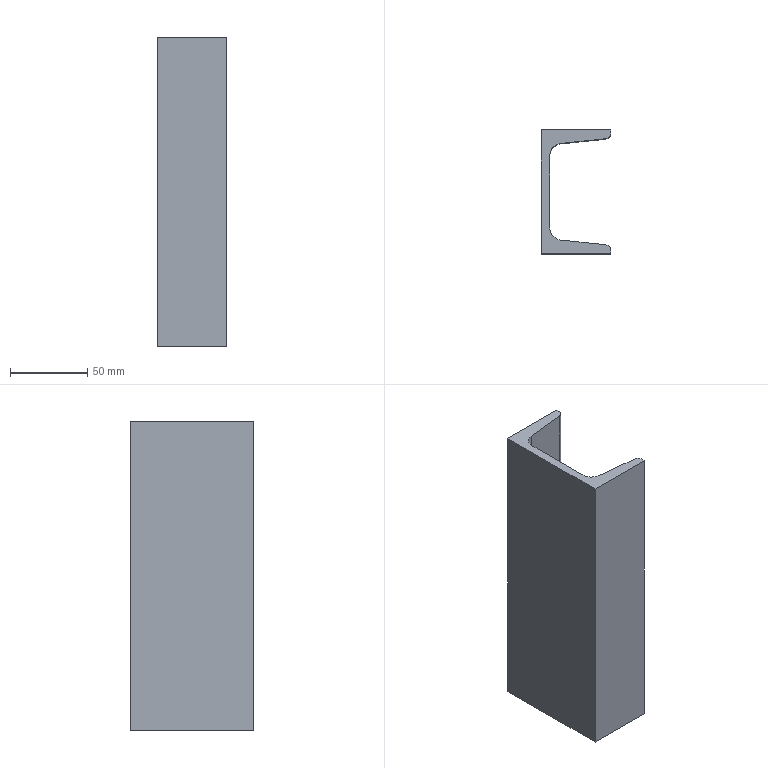Part | STEP file | ISO 657_11 CH 80 x 8 1784900614284 | 1 solid | 14 faces | box 45 x 80 x 200 mm | volume 209713 mm3 | plane 10 | cylinder 4 | commonest cylinder face diameters 8 x2 16 x2
STEP:
#1=CARTESIAN_POINT('',(4.07,-23.221,200.));
#2=VERTEX_POINT('',#1);
#3=CARTESIAN_POINT('',(11.234,-31.177,200.));
#4=VERTEX_POINT('',#3);
#5=CARTESIAN_POINT('',(12.07,-23.221,200.));
#6=DIRECTION('',(0.,0.,1.));
#7=DIRECTION('',(-1.,0.,0.));
#8=AXIS2_PLACEMENT_3D('',#5,#6,#7);
#9=CIRCLE('',#8,8.);
#10=EDGE_CURVE('',#2,#4,#9,.T.);
#11=ORIENTED_EDGE('',*,*,#10,.T.);
#12=CARTESIAN_POINT('',(11.234,-31.177,0.));
#13=VERTEX_POINT('',#12);
#14=CARTESIAN_POINT('',(11.234,-31.177,0.));
#15=DIRECTION('',(0.,0.,1.));
#16=VECTOR('',#15,10.);
#17=LINE('',#14,#16);
#18=EDGE_CURVE('',#13,#4,#17,.T.);
#19=ORIENTED_EDGE('',*,*,#18,.F.);
#20=CARTESIAN_POINT('',(4.07,-23.221,0.));
#21=VERTEX_POINT('',#20);
#22=CARTESIAN_POINT('',(12.07,-23.221,0.));
#23=DIRECTION('',(0.,0.,1.));
#24=DIRECTION('',(-1.,0.,0.));
#25=AXIS2_PLACEMENT_3D('',#22,#23,#24);
#26=CIRCLE('',#25,8.);
#27=EDGE_CURVE('',#21,#13,#26,.T.);
#28=ORIENTED_EDGE('',*,*,#27,.F.);
#29=CARTESIAN_POINT('',(4.07,-23.221,0.));
#30=DIRECTION('',(0.,0.,1.));
#31=VECTOR('',#30,10.);
#32=LINE('',#29,#31);
#33=EDGE_CURVE('',#21,#2,#32,.T.);
#34=ORIENTED_EDGE('',*,*,#33,.T.);
#35=EDGE_LOOP('',(#11,#19,#28,#34));
#36=FACE_OUTER_BOUND('',#35,.T.);
#37=CARTESIAN_POINT('',(12.07,-23.221,0.));
#38=DIRECTION('',(0.,0.,1.));
#39=DIRECTION('',(-1.,0.,0.));
#40=AXIS2_PLACEMENT_3D('',#37,#38,#39);
#41=CYLINDRICAL_SURFACE('',#40,8.);
#42=ADVANCED_FACE('',(#36),#41,.F.);
#43=CARTESIAN_POINT('',(39.988,-34.199,200.));
#44=VERTEX_POINT('',#43);
#45=CARTESIAN_POINT('',(14.478,-31.518,200.));
#46=DIRECTION('',(0.9945,-0.1045,0.));
#47=VECTOR('',#46,10.);
#48=LINE('',#45,#47);
#49=EDGE_CURVE('',#4,#44,#48,.T.);
#50=ORIENTED_EDGE('',*,*,#49,.T.);
#51=CARTESIAN_POINT('',(39.988,-34.199,0.));
#52=VERTEX_POINT('',#51);
#53=CARTESIAN_POINT('',(39.988,-34.199,0.));
#54=DIRECTION('',(0.,0.,1.));
#55=VECTOR('',#54,10.);
#56=LINE('',#53,#55);
#57=EDGE_CURVE('',#52,#44,#56,.T.);
#58=ORIENTED_EDGE('',*,*,#57,.F.);
#59=CARTESIAN_POINT('',(14.478,-31.518,0.));
#60=DIRECTION('',(0.9945,-0.1045,0.));
#61=VECTOR('',#60,10.);
#62=LINE('',#59,#61);
#63=EDGE_CURVE('',#13,#52,#62,.T.);
#64=ORIENTED_EDGE('',*,*,#63,.F.);
#65=ORIENTED_EDGE('',*,*,#18,.T.);
#66=EDGE_LOOP('',(#50,#58,#64,#65));
#67=FACE_OUTER_BOUND('',#66,.T.);
#68=CARTESIAN_POINT('',(11.234,-31.177,0.));
#69=DIRECTION('',(0.1045,0.9945,0.));
#70=DIRECTION('',(0.,0.,1.));
#71=AXIS2_PLACEMENT_3D('',#68,#69,#70);
#72=PLANE('',#71);
#73=ADVANCED_FACE('',(#67),#72,.T.);
#74=CARTESIAN_POINT('',(43.57,-38.177,200.));
#75=VERTEX_POINT('',#74);
#76=CARTESIAN_POINT('',(39.57,-38.177,200.));
#77=DIRECTION('',(0.,0.,-1.));
#78=DIRECTION('',(-1.,0.,0.));
#79=AXIS2_PLACEMENT_3D('',#76,#77,#78);
#80=CIRCLE('',#79,4.);
#81=EDGE_CURVE('',#44,#75,#80,.T.);
#82=ORIENTED_EDGE('',*,*,#81,.T.);
#83=CARTESIAN_POINT('',(43.57,-38.177,0.));
#84=VERTEX_POINT('',#83);
#85=CARTESIAN_POINT('',(43.57,-38.177,0.));
#86=DIRECTION('',(0.,0.,1.));
#87=VECTOR('',#86,10.);
#88=LINE('',#85,#87);
#89=EDGE_CURVE('',#84,#75,#88,.T.);
#90=ORIENTED_EDGE('',*,*,#89,.F.);
#91=CARTESIAN_POINT('',(39.57,-38.177,0.));
#92=DIRECTION('',(0.,0.,-1.));
#93=DIRECTION('',(-1.,0.,0.));
#94=AXIS2_PLACEMENT_3D('',#91,#92,#93);
#95=CIRCLE('',#94,4.);
#96=EDGE_CURVE('',#52,#84,#95,.T.);
#97=ORIENTED_EDGE('',*,*,#96,.F.);
#98=ORIENTED_EDGE('',*,*,#57,.T.);
#99=EDGE_LOOP('',(#82,#90,#97,#98));
#100=FACE_OUTER_BOUND('',#99,.T.);
#101=CARTESIAN_POINT('',(39.57,-38.177,0.));
#102=DIRECTION('',(0.,0.,1.));
#103=DIRECTION('',(-1.,0.,0.));
#104=AXIS2_PLACEMENT_3D('',#101,#102,#103);
#105=CYLINDRICAL_SURFACE('',#104,4.);
#106=ADVANCED_FACE('',(#100),#105,.T.);
#107=CARTESIAN_POINT('',(43.57,-40.,200.));
#108=VERTEX_POINT('',#107);
#109=CARTESIAN_POINT('',(43.57,-19.089,200.));
#110=DIRECTION('',(0.,-1.,0.));
#111=VECTOR('',#110,10.);
#112=LINE('',#109,#111);
#113=EDGE_CURVE('',#75,#108,#112,.T.);
#114=ORIENTED_EDGE('',*,*,#113,.T.);
#115=CARTESIAN_POINT('',(43.57,-40.,0.));
#116=VERTEX_POINT('',#115);
#117=CARTESIAN_POINT('',(43.57,-40.,0.));
#118=DIRECTION('',(0.,0.,1.));
#119=VECTOR('',#118,10.);
#120=LINE('',#117,#119);
#121=EDGE_CURVE('',#116,#108,#120,.T.);
#122=ORIENTED_EDGE('',*,*,#121,.F.);
#123=CARTESIAN_POINT('',(43.57,-19.089,0.));
#124=DIRECTION('',(0.,-1.,0.));
#125=VECTOR('',#124,10.);
#126=LINE('',#123,#125);
#127=EDGE_CURVE('',#84,#116,#126,.T.);
#128=ORIENTED_EDGE('',*,*,#127,.F.);
#129=ORIENTED_EDGE('',*,*,#89,.T.);
#130=EDGE_LOOP('',(#114,#122,#128,#129));
#131=FACE_OUTER_BOUND('',#130,.T.);
#132=CARTESIAN_POINT('',(43.57,-38.177,0.));
#133=DIRECTION('',(1.,0.,0.));
#134=DIRECTION('',(0.,0.,-1.));
#135=AXIS2_PLACEMENT_3D('',#132,#133,#134);
#136=PLANE('',#135);
#137=ADVANCED_FACE('',(#131),#136,.T.);
#138=CARTESIAN_POINT('',(-1.43,-40.,200.));
#139=VERTEX_POINT('',#138);
#140=CARTESIAN_POINT('',(32.32,-40.,200.));
#141=DIRECTION('',(-1.,0.,0.));
#142=VECTOR('',#141,10.);
#143=LINE('',#140,#142);
#144=EDGE_CURVE('',#108,#139,#143,.T.);
#145=ORIENTED_EDGE('',*,*,#144,.T.);
#146=CARTESIAN_POINT('',(-1.43,-40.,0.));
#147=VERTEX_POINT('',#146);
#148=CARTESIAN_POINT('',(-1.43,-40.,0.));
#149=DIRECTION('',(0.,0.,1.));
#150=VECTOR('',#149,10.);
#151=LINE('',#148,#150);
#152=EDGE_CURVE('',#147,#139,#151,.T.);
#153=ORIENTED_EDGE('',*,*,#152,.F.);
#154=CARTESIAN_POINT('',(32.32,-40.,0.));
#155=DIRECTION('',(-1.,0.,0.));
#156=VECTOR('',#155,10.);
#157=LINE('',#154,#156);
#158=EDGE_CURVE('',#116,#147,#157,.T.);
#159=ORIENTED_EDGE('',*,*,#158,.F.);
#160=ORIENTED_EDGE('',*,*,#121,.T.);
#161=EDGE_LOOP('',(#145,#153,#159,#160));
#162=FACE_OUTER_BOUND('',#161,.T.);
#163=CARTESIAN_POINT('',(43.57,-40.,0.));
#164=DIRECTION('',(0.,-1.,0.));
#165=DIRECTION('',(0.,0.,-1.));
#166=AXIS2_PLACEMENT_3D('',#163,#164,#165);
#167=PLANE('',#166);
#168=ADVANCED_FACE('',(#162),#167,.T.);
#169=CARTESIAN_POINT('',(-1.43,40.,200.));
#170=VERTEX_POINT('',#169);
#171=CARTESIAN_POINT('',(-1.43,0.,200.));
#172=DIRECTION('',(0.,1.,0.));
#173=VECTOR('',#172,10.);
#174=LINE('',#171,#173);
#175=EDGE_CURVE('',#139,#170,#174,.T.);
#176=ORIENTED_EDGE('',*,*,#175,.T.);
#177=CARTESIAN_POINT('',(-1.43,40.,0.));
#178=VERTEX_POINT('',#177);
#179=CARTESIAN_POINT('',(-1.43,40.,0.));
#180=DIRECTION('',(0.,0.,1.));
#181=VECTOR('',#180,10.);
#182=LINE('',#179,#181);
#183=EDGE_CURVE('',#178,#170,#182,.T.);
#184=ORIENTED_EDGE('',*,*,#183,.F.);
#185=CARTESIAN_POINT('',(-1.43,0.,0.));
#186=DIRECTION('',(0.,1.,0.));
#187=VECTOR('',#186,10.);
#188=LINE('',#185,#187);
#189=EDGE_CURVE('',#147,#178,#188,.T.);
#190=ORIENTED_EDGE('',*,*,#189,.F.);
#191=ORIENTED_EDGE('',*,*,#152,.T.);
#192=EDGE_LOOP('',(#176,#184,#190,#191));
#193=FACE_OUTER_BOUND('',#192,.T.);
#194=CARTESIAN_POINT('',(-1.43,0.,0.));
#195=DIRECTION('',(-1.,0.,0.));
#196=DIRECTION('',(0.,0.,1.));
#197=AXIS2_PLACEMENT_3D('',#194,#195,#196);
#198=PLANE('',#197);
#199=ADVANCED_FACE('',(#193),#198,.T.);
#200=CARTESIAN_POINT('',(43.57,40.,200.));
#201=VERTEX_POINT('',#200);
#202=CARTESIAN_POINT('',(9.82,40.,200.));
#203=DIRECTION('',(1.,0.,0.));
#204=VECTOR('',#203,10.);
#205=LINE('',#202,#204);
#206=EDGE_CURVE('',#170,#201,#205,.T.);
#207=ORIENTED_EDGE('',*,*,#206,.T.);
#208=CARTESIAN_POINT('',(43.57,40.,0.));
#209=VERTEX_POINT('',#208);
#210=CARTESIAN_POINT('',(43.57,40.,0.));
#211=DIRECTION('',(0.,0.,1.));
#212=VECTOR('',#211,10.);
#213=LINE('',#210,#212);
#214=EDGE_CURVE('',#209,#201,#213,.T.);
#215=ORIENTED_EDGE('',*,*,#214,.F.);
#216=CARTESIAN_POINT('',(9.82,40.,0.));
#217=DIRECTION('',(1.,0.,0.));
#218=VECTOR('',#217,10.);
#219=LINE('',#216,#218);
#220=EDGE_CURVE('',#178,#209,#219,.T.);
#221=ORIENTED_EDGE('',*,*,#220,.F.);
#222=ORIENTED_EDGE('',*,*,#183,.T.);
#223=EDGE_LOOP('',(#207,#215,#221,#222));
#224=FACE_OUTER_BOUND('',#223,.T.);
#225=CARTESIAN_POINT('',(-1.43,40.,0.));
#226=DIRECTION('',(0.,1.,0.));
#227=DIRECTION('',(0.,0.,1.));
#228=AXIS2_PLACEMENT_3D('',#225,#226,#227);
#229=PLANE('',#228);
#230=ADVANCED_FACE('',(#224),#229,.T.);
#231=CARTESIAN_POINT('',(43.57,38.177,200.));
#232=VERTEX_POINT('',#231);
#233=CARTESIAN_POINT('',(43.57,20.,200.));
#234=DIRECTION('',(0.,-1.,0.));
#235=VECTOR('',#234,10.);
#236=LINE('',#233,#235);
#237=EDGE_CURVE('',#201,#232,#236,.T.);
#238=ORIENTED_EDGE('',*,*,#237,.T.);
#239=CARTESIAN_POINT('',(43.57,38.177,0.));
#240=VERTEX_POINT('',#239);
#241=CARTESIAN_POINT('',(43.57,38.177,0.));
#242=DIRECTION('',(0.,0.,1.));
#243=VECTOR('',#242,10.);
#244=LINE('',#241,#243);
#245=EDGE_CURVE('',#240,#232,#244,.T.);
#246=ORIENTED_EDGE('',*,*,#245,.F.);
#247=CARTESIAN_POINT('',(43.57,20.,0.));
#248=DIRECTION('',(0.,-1.,0.));
#249=VECTOR('',#248,10.);
#250=LINE('',#247,#249);
#251=EDGE_CURVE('',#209,#240,#250,.T.);
#252=ORIENTED_EDGE('',*,*,#251,.F.);
#253=ORIENTED_EDGE('',*,*,#214,.T.);
#254=EDGE_LOOP('',(#238,#246,#252,#253));
#255=FACE_OUTER_BOUND('',#254,.T.);
#256=CARTESIAN_POINT('',(43.57,40.,0.));
#257=DIRECTION('',(1.,0.,0.));
#258=DIRECTION('',(0.,0.,-1.));
#259=AXIS2_PLACEMENT_3D('',#256,#257,#258);
#260=PLANE('',#259);
#261=ADVANCED_FACE('',(#255),#260,.T.);
#262=CARTESIAN_POINT('',(39.988,34.199,200.));
#263=VERTEX_POINT('',#262);
#264=CARTESIAN_POINT('',(39.57,38.177,200.));
#265=DIRECTION('',(0.,0.,-1.));
#266=DIRECTION('',(-0.1045,0.9945,0.));
#267=AXIS2_PLACEMENT_3D('',#264,#265,#266);
#268=CIRCLE('',#267,4.);
#269=EDGE_CURVE('',#232,#263,#268,.T.);
#270=ORIENTED_EDGE('',*,*,#269,.T.);
#271=CARTESIAN_POINT('',(39.988,34.199,0.));
#272=VERTEX_POINT('',#271);
#273=CARTESIAN_POINT('',(39.988,34.199,0.));
#274=DIRECTION('',(0.,0.,1.));
#275=VECTOR('',#274,10.);
#276=LINE('',#273,#275);
#277=EDGE_CURVE('',#272,#263,#276,.T.);
#278=ORIENTED_EDGE('',*,*,#277,.F.);
#279=CARTESIAN_POINT('',(39.57,38.177,0.));
#280=DIRECTION('',(0.,0.,-1.));
#281=DIRECTION('',(-0.1045,0.9945,0.));
#282=AXIS2_PLACEMENT_3D('',#279,#280,#281);
#283=CIRCLE('',#282,4.);
#284=EDGE_CURVE('',#240,#272,#283,.T.);
#285=ORIENTED_EDGE('',*,*,#284,.F.);
#286=ORIENTED_EDGE('',*,*,#245,.T.);
#287=EDGE_LOOP('',(#270,#278,#285,#286));
#288=FACE_OUTER_BOUND('',#287,.T.);
#289=CARTESIAN_POINT('',(39.57,38.177,0.));
#290=DIRECTION('',(0.,0.,1.));
#291=DIRECTION('',(-0.1045,0.9945,0.));
#292=AXIS2_PLACEMENT_3D('',#289,#290,#291);
#293=CYLINDRICAL_SURFACE('',#292,4.);
#294=ADVANCED_FACE('',(#288),#293,.T.);
#295=CARTESIAN_POINT('',(11.234,31.177,200.));
#296=VERTEX_POINT('',#295);
#297=CARTESIAN_POINT('',(28.855,33.029,200.));
#298=DIRECTION('',(-0.9945,-0.1045,0.));
#299=VECTOR('',#298,10.);
#300=LINE('',#297,#299);
#301=EDGE_CURVE('',#263,#296,#300,.T.);
#302=ORIENTED_EDGE('',*,*,#301,.T.);
#303=CARTESIAN_POINT('',(11.234,31.177,0.));
#304=VERTEX_POINT('',#303);
#305=CARTESIAN_POINT('',(11.234,31.177,0.));
#306=DIRECTION('',(0.,0.,1.));
#307=VECTOR('',#306,10.);
#308=LINE('',#305,#307);
#309=EDGE_CURVE('',#304,#296,#308,.T.);
#310=ORIENTED_EDGE('',*,*,#309,.F.);
#311=CARTESIAN_POINT('',(28.855,33.029,0.));
#312=DIRECTION('',(-0.9945,-0.1045,0.));
#313=VECTOR('',#312,10.);
#314=LINE('',#311,#313);
#315=EDGE_CURVE('',#272,#304,#314,.T.);
#316=ORIENTED_EDGE('',*,*,#315,.F.);
#317=ORIENTED_EDGE('',*,*,#277,.T.);
#318=EDGE_LOOP('',(#302,#310,#316,#317));
#319=FACE_OUTER_BOUND('',#318,.T.);
#320=CARTESIAN_POINT('',(39.988,34.199,0.));
#321=DIRECTION('',(0.1045,-0.9945,0.));
#322=DIRECTION('',(0.,0.,-1.));
#323=AXIS2_PLACEMENT_3D('',#320,#321,#322);
#324=PLANE('',#323);
#325=ADVANCED_FACE('',(#319),#324,.T.);
#326=CARTESIAN_POINT('',(4.07,23.221,200.));
#327=VERTEX_POINT('',#326);
#328=CARTESIAN_POINT('',(12.07,23.221,200.));
#329=DIRECTION('',(0.,0.,1.));
#330=DIRECTION('',(-0.1045,0.9945,0.));
#331=AXIS2_PLACEMENT_3D('',#328,#329,#330);
#332=CIRCLE('',#331,8.);
#333=EDGE_CURVE('',#296,#327,#332,.T.);
#334=ORIENTED_EDGE('',*,*,#333,.T.);
#335=CARTESIAN_POINT('',(4.07,23.221,0.));
#336=VERTEX_POINT('',#335);
#337=CARTESIAN_POINT('',(4.07,23.221,0.));
#338=DIRECTION('',(0.,0.,1.));
#339=VECTOR('',#338,10.);
#340=LINE('',#337,#339);
#341=EDGE_CURVE('',#336,#327,#340,.T.);
#342=ORIENTED_EDGE('',*,*,#341,.F.);
#343=CARTESIAN_POINT('',(12.07,23.221,0.));
#344=DIRECTION('',(0.,0.,1.));
#345=DIRECTION('',(-0.1045,0.9945,0.));
#346=AXIS2_PLACEMENT_3D('',#343,#344,#345);
#347=CIRCLE('',#346,8.);
#348=EDGE_CURVE('',#304,#336,#347,.T.);
#349=ORIENTED_EDGE('',*,*,#348,.F.);
#350=ORIENTED_EDGE('',*,*,#309,.T.);
#351=EDGE_LOOP('',(#334,#342,#349,#350));
#352=FACE_OUTER_BOUND('',#351,.T.);
#353=CARTESIAN_POINT('',(12.07,23.221,0.));
#354=DIRECTION('',(0.,0.,1.));
#355=DIRECTION('',(-0.1045,0.9945,0.));
#356=AXIS2_PLACEMENT_3D('',#353,#354,#355);
#357=CYLINDRICAL_SURFACE('',#356,8.);
#358=ADVANCED_FACE('',(#352),#357,.F.);
#359=CARTESIAN_POINT('',(4.07,0.,200.));
#360=DIRECTION('',(0.,-1.,0.));
#361=VECTOR('',#360,10.);
#362=LINE('',#359,#361);
#363=EDGE_CURVE('',#327,#2,#362,.T.);
#364=ORIENTED_EDGE('',*,*,#363,.T.);
#365=ORIENTED_EDGE('',*,*,#33,.F.);
#366=CARTESIAN_POINT('',(4.07,0.,0.));
#367=DIRECTION('',(0.,-1.,0.));
#368=VECTOR('',#367,10.);
#369=LINE('',#366,#368);
#370=EDGE_CURVE('',#336,#21,#369,.T.);
#371=ORIENTED_EDGE('',*,*,#370,.F.);
#372=ORIENTED_EDGE('',*,*,#341,.T.);
#373=EDGE_LOOP('',(#364,#365,#371,#372));
#374=FACE_OUTER_BOUND('',#373,.T.);
#375=CARTESIAN_POINT('',(4.07,0.,0.));
#376=DIRECTION('',(1.,0.,0.));
#377=DIRECTION('',(0.,0.,-1.));
#378=AXIS2_PLACEMENT_3D('',#375,#376,#377);
#379=PLANE('',#378);
#380=ADVANCED_FACE('',(#374),#379,.T.);
#381=ORIENTED_EDGE('',*,*,#220,.T.);
#382=ORIENTED_EDGE('',*,*,#251,.T.);
#383=ORIENTED_EDGE('',*,*,#284,.T.);
#384=ORIENTED_EDGE('',*,*,#315,.T.);
#385=ORIENTED_EDGE('',*,*,#348,.T.);
#386=ORIENTED_EDGE('',*,*,#370,.T.);
#387=ORIENTED_EDGE('',*,*,#27,.T.);
#388=ORIENTED_EDGE('',*,*,#63,.T.);
#389=ORIENTED_EDGE('',*,*,#96,.T.);
#390=ORIENTED_EDGE('',*,*,#127,.T.);
#391=ORIENTED_EDGE('',*,*,#158,.T.);
#392=ORIENTED_EDGE('',*,*,#189,.T.);
#393=EDGE_LOOP('',(#381,#382,#383,#384,#385,#386,#387,#388,#389,#390,#391,#392));
#394=FACE_OUTER_BOUND('',#393,.T.);
#395=CARTESIAN_POINT('',(21.07,0.,0.));
#396=DIRECTION('',(0.,0.,1.));
#397=DIRECTION('',(1.,0.,0.));
#398=AXIS2_PLACEMENT_3D('',#395,#396,#397);
#399=PLANE('',#398);
#400=ADVANCED_FACE('',(#394),#399,.F.);
#401=ORIENTED_EDGE('',*,*,#206,.F.);
#402=ORIENTED_EDGE('',*,*,#175,.F.);
#403=ORIENTED_EDGE('',*,*,#144,.F.);
#404=ORIENTED_EDGE('',*,*,#113,.F.);
#405=ORIENTED_EDGE('',*,*,#81,.F.);
#406=ORIENTED_EDGE('',*,*,#49,.F.);
#407=ORIENTED_EDGE('',*,*,#10,.F.);
#408=ORIENTED_EDGE('',*,*,#363,.F.);
#409=ORIENTED_EDGE('',*,*,#333,.F.);
#410=ORIENTED_EDGE('',*,*,#301,.F.);
#411=ORIENTED_EDGE('',*,*,#269,.F.);
#412=ORIENTED_EDGE('',*,*,#237,.F.);
#413=EDGE_LOOP('',(#401,#402,#403,#404,#405,#406,#407,#408,#409,#410,#411,#412));
#414=FACE_OUTER_BOUND('',#413,.T.);
#415=CARTESIAN_POINT('',(21.07,0.,200.));
#416=DIRECTION('',(0.,0.,1.));
#417=DIRECTION('',(1.,0.,0.));
#418=AXIS2_PLACEMENT_3D('',#415,#416,#417);
#419=PLANE('',#418);
#420=ADVANCED_FACE('',(#414),#419,.T.);
#421=CLOSED_SHELL('',(#42,#73,#106,#137,#168,#199,#230,#261,#294,#325,#358,#380,#400,#420));
#422=MANIFOLD_SOLID_BREP('',#421);
#423=(LENGTH_UNIT()NAMED_UNIT(*)SI_UNIT(.MILLI.,.METRE.));
#424=UNCERTAINTY_MEASURE_WITH_UNIT(LENGTH_MEASURE(0.01),#423,'','');
#425=(NAMED_UNIT(*)PLANE_ANGLE_UNIT()SI_UNIT($,.RADIAN.));
#426=(NAMED_UNIT(*)SI_UNIT($,.STERADIAN.)SOLID_ANGLE_UNIT());
#427=(GEOMETRIC_REPRESENTATION_CONTEXT(3)GLOBAL_UNCERTAINTY_ASSIGNED_CONTEXT((#424))GLOBAL_UNIT_ASSIGNED_CONTEXT((#423,#425,#426))REPRESENTATION_CONTEXT('',''));
#428=ADVANCED_BREP_SHAPE_REPRESENTATION('',(#422),#427);